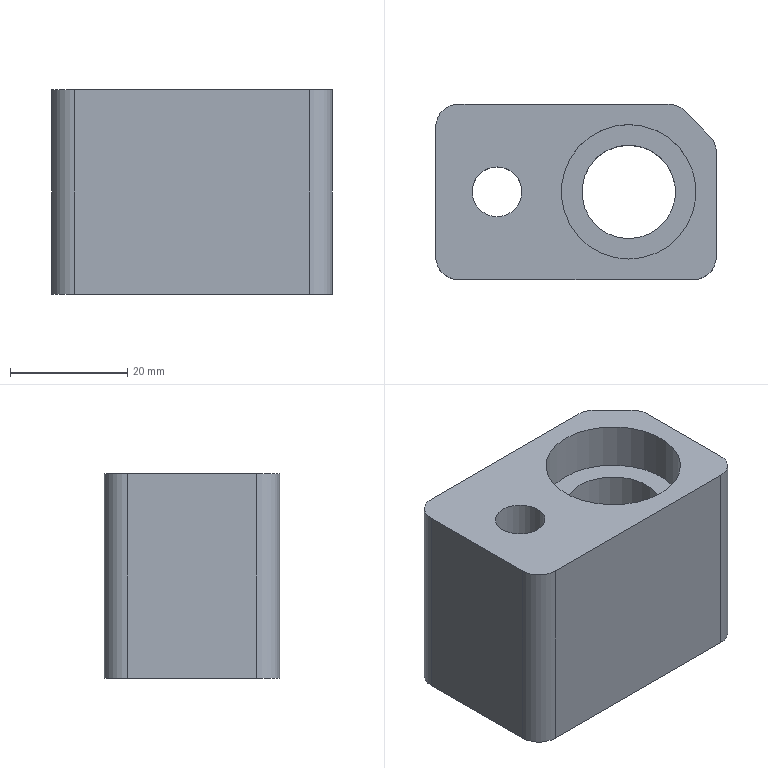Part | NX | features 7 2 | 1 solid | 18 faces | box 48 x 30 x 35 mm | volume 36880 mm3 | plane 9 | cylinder 9 | commonest cylinder face diameters 8 x5 8.5 x1 14.5 x1 16 x1 23 x1
STEP:
#1=CARTESIAN_POINT('',(21.306,11.5,91.));
#2=VERTEX_POINT('',#1);
#3=CARTESIAN_POINT('',(21.306,0.,91.));
#4=DIRECTION('',(0.,0.,-1.));
#5=DIRECTION('',(0.,1.,0.));
#6=AXIS2_PLACEMENT_3D('',#3,#4,#5);
#7=CIRCLE('',#6,11.5);
#8=EDGE_CURVE('',#2,#2,#7,.T.);
#9=ORIENTED_EDGE('',*,*,#8,.T.);
#10=EDGE_LOOP('',(#9));
#11=FACE_BOUND('',#10,.T.);
#12=CARTESIAN_POINT('',(-7.694,-15.,91.));
#13=VERTEX_POINT('',#12);
#14=CARTESIAN_POINT('',(32.306,-15.,91.));
#15=VERTEX_POINT('',#14);
#16=CARTESIAN_POINT('',(21.306,-15.,91.));
#17=DIRECTION('',(1.,0.,0.));
#18=VECTOR('',#17,1000.);
#19=LINE('',#16,#18);
#20=EDGE_CURVE('',#13,#15,#19,.T.);
#21=ORIENTED_EDGE('',*,*,#20,.T.);
#22=CARTESIAN_POINT('',(36.306,-11.,91.));
#23=VERTEX_POINT('',#22);
#24=CARTESIAN_POINT('',(32.306,-11.,91.));
#25=DIRECTION('',(0.,0.,-1.));
#26=DIRECTION('',(0.,1.,0.));
#27=AXIS2_PLACEMENT_3D('',#24,#25,#26);
#28=CIRCLE('',#27,4.);
#29=EDGE_CURVE('',#23,#15,#28,.T.);
#30=ORIENTED_EDGE('',*,*,#29,.F.);
#31=CARTESIAN_POINT('',(36.306,6.707,91.));
#32=VERTEX_POINT('',#31);
#33=CARTESIAN_POINT('',(36.306,0.,91.));
#34=DIRECTION('',(0.,1.,0.));
#35=VECTOR('',#34,1000.);
#36=LINE('',#33,#35);
#37=EDGE_CURVE('',#23,#32,#36,.T.);
#38=ORIENTED_EDGE('',*,*,#37,.T.);
#39=CARTESIAN_POINT('',(35.135,9.536,91.));
#40=VERTEX_POINT('',#39);
#41=CARTESIAN_POINT('',(32.306,6.707,91.));
#42=DIRECTION('',(0.,0.,-1.));
#43=DIRECTION('',(0.,1.,0.));
#44=AXIS2_PLACEMENT_3D('',#41,#42,#43);
#45=CIRCLE('',#44,4.);
#46=EDGE_CURVE('',#40,#32,#45,.T.);
#47=ORIENTED_EDGE('',*,*,#46,.F.);
#48=CARTESIAN_POINT('',(30.842,13.828,91.));
#49=VERTEX_POINT('',#48);
#50=CARTESIAN_POINT('',(31.738,12.932,91.));
#51=DIRECTION('',(0.7071,-0.7071,0.));
#52=VECTOR('',#51,1000.);
#53=LINE('',#50,#52);
#54=EDGE_CURVE('',#49,#40,#53,.T.);
#55=ORIENTED_EDGE('',*,*,#54,.F.);
#56=CARTESIAN_POINT('',(28.013,15.,91.));
#57=VERTEX_POINT('',#56);
#58=CARTESIAN_POINT('',(28.013,11.,91.));
#59=DIRECTION('',(0.,0.,-1.));
#60=DIRECTION('',(0.,1.,0.));
#61=AXIS2_PLACEMENT_3D('',#58,#59,#60);
#62=CIRCLE('',#61,4.);
#63=EDGE_CURVE('',#57,#49,#62,.T.);
#64=ORIENTED_EDGE('',*,*,#63,.F.);
#65=CARTESIAN_POINT('',(-7.694,15.,91.));
#66=VERTEX_POINT('',#65);
#67=CARTESIAN_POINT('',(21.306,15.,91.));
#68=DIRECTION('',(-1.,0.,0.));
#69=VECTOR('',#68,1000.);
#70=LINE('',#67,#69);
#71=EDGE_CURVE('',#57,#66,#70,.T.);
#72=ORIENTED_EDGE('',*,*,#71,.T.);
#73=CARTESIAN_POINT('',(-11.694,11.,91.));
#74=VERTEX_POINT('',#73);
#75=CARTESIAN_POINT('',(-7.694,11.,91.));
#76=DIRECTION('',(0.,0.,-1.));
#77=DIRECTION('',(0.,1.,0.));
#78=AXIS2_PLACEMENT_3D('',#75,#76,#77);
#79=CIRCLE('',#78,4.);
#80=EDGE_CURVE('',#74,#66,#79,.T.);
#81=ORIENTED_EDGE('',*,*,#80,.F.);
#82=CARTESIAN_POINT('',(-11.694,-11.,91.));
#83=VERTEX_POINT('',#82);
#84=CARTESIAN_POINT('',(-11.694,0.,91.));
#85=DIRECTION('',(0.,-1.,0.));
#86=VECTOR('',#85,1000.);
#87=LINE('',#84,#86);
#88=EDGE_CURVE('',#74,#83,#87,.T.);
#89=ORIENTED_EDGE('',*,*,#88,.T.);
#90=CARTESIAN_POINT('',(-7.694,-11.,91.));
#91=DIRECTION('',(0.,0.,-1.));
#92=DIRECTION('',(0.,1.,0.));
#93=AXIS2_PLACEMENT_3D('',#90,#91,#92);
#94=CIRCLE('',#93,4.);
#95=EDGE_CURVE('',#13,#83,#94,.T.);
#96=ORIENTED_EDGE('',*,*,#95,.F.);
#97=EDGE_LOOP('',(#21,#30,#38,#47,#55,#64,#72,#81,#89,#96));
#98=FACE_BOUND('',#97,.T.);
#99=CARTESIAN_POINT('',(-1.194,4.25,91.));
#100=VERTEX_POINT('',#99);
#101=CARTESIAN_POINT('',(-1.194,0.,91.));
#102=DIRECTION('',(0.,0.,1.));
#103=DIRECTION('',(0.,1.,0.));
#104=AXIS2_PLACEMENT_3D('',#101,#102,#103);
#105=CIRCLE('',#104,4.25);
#106=EDGE_CURVE('',#100,#100,#105,.T.);
#107=ORIENTED_EDGE('',*,*,#106,.F.);
#108=EDGE_LOOP('',(#107));
#109=FACE_BOUND('',#108,.T.);
#110=CARTESIAN_POINT('',(18.806,0.,91.));
#111=DIRECTION('',(0.,0.,1.));
#112=DIRECTION('',(0.,-1.,0.));
#113=AXIS2_PLACEMENT_3D('',#110,#111,#112);
#114=PLANE('',#113);
#115=ADVANCED_FACE('',(#11,#98,#109),#114,.T.);
#116=CARTESIAN_POINT('',(21.306,-8.,56.));
#117=VERTEX_POINT('',#116);
#118=CARTESIAN_POINT('',(21.306,0.,56.));
#119=DIRECTION('',(0.,0.,1.));
#120=DIRECTION('',(0.,-1.,0.));
#121=AXIS2_PLACEMENT_3D('',#118,#119,#120);
#122=CIRCLE('',#121,8.);
#123=EDGE_CURVE('',#117,#117,#122,.T.);
#124=ORIENTED_EDGE('',*,*,#123,.T.);
#125=EDGE_LOOP('',(#124));
#126=FACE_BOUND('',#125,.T.);
#127=CARTESIAN_POINT('',(-1.194,-7.25,56.));
#128=VERTEX_POINT('',#127);
#129=CARTESIAN_POINT('',(-1.194,0.,56.));
#130=DIRECTION('',(0.,0.,1.));
#131=DIRECTION('',(0.,-1.,0.));
#132=AXIS2_PLACEMENT_3D('',#129,#130,#131);
#133=CIRCLE('',#132,7.25);
#134=EDGE_CURVE('',#128,#128,#133,.T.);
#135=ORIENTED_EDGE('',*,*,#134,.T.);
#136=EDGE_LOOP('',(#135));
#137=FACE_BOUND('',#136,.T.);
#138=CARTESIAN_POINT('',(-11.694,-11.,56.));
#139=VERTEX_POINT('',#138);
#140=CARTESIAN_POINT('',(-11.694,11.,56.));
#141=VERTEX_POINT('',#140);
#142=CARTESIAN_POINT('',(-11.694,0.,56.));
#143=DIRECTION('',(0.,1.,0.));
#144=VECTOR('',#143,1000.);
#145=LINE('',#142,#144);
#146=EDGE_CURVE('',#139,#141,#145,.T.);
#147=ORIENTED_EDGE('',*,*,#146,.T.);
#148=CARTESIAN_POINT('',(-7.694,15.,56.));
#149=VERTEX_POINT('',#148);
#150=CARTESIAN_POINT('',(-7.694,11.,56.));
#151=DIRECTION('',(0.,0.,1.));
#152=DIRECTION('',(0.,-1.,0.));
#153=AXIS2_PLACEMENT_3D('',#150,#151,#152);
#154=CIRCLE('',#153,4.);
#155=EDGE_CURVE('',#149,#141,#154,.T.);
#156=ORIENTED_EDGE('',*,*,#155,.F.);
#157=CARTESIAN_POINT('',(28.013,15.,56.));
#158=VERTEX_POINT('',#157);
#159=CARTESIAN_POINT('',(21.306,15.,56.));
#160=DIRECTION('',(1.,0.,0.));
#161=VECTOR('',#160,1000.);
#162=LINE('',#159,#161);
#163=EDGE_CURVE('',#149,#158,#162,.T.);
#164=ORIENTED_EDGE('',*,*,#163,.T.);
#165=CARTESIAN_POINT('',(30.842,13.828,56.));
#166=VERTEX_POINT('',#165);
#167=CARTESIAN_POINT('',(28.013,11.,56.));
#168=DIRECTION('',(0.,0.,1.));
#169=DIRECTION('',(0.,-1.,0.));
#170=AXIS2_PLACEMENT_3D('',#167,#168,#169);
#171=CIRCLE('',#170,4.);
#172=EDGE_CURVE('',#166,#158,#171,.T.);
#173=ORIENTED_EDGE('',*,*,#172,.F.);
#174=CARTESIAN_POINT('',(35.135,9.536,56.));
#175=VERTEX_POINT('',#174);
#176=CARTESIAN_POINT('',(28.988,15.682,56.));
#177=DIRECTION('',(-0.7071,0.7071,0.));
#178=VECTOR('',#177,1000.);
#179=LINE('',#176,#178);
#180=EDGE_CURVE('',#175,#166,#179,.T.);
#181=ORIENTED_EDGE('',*,*,#180,.F.);
#182=CARTESIAN_POINT('',(36.306,6.707,56.));
#183=VERTEX_POINT('',#182);
#184=CARTESIAN_POINT('',(32.306,6.707,56.));
#185=DIRECTION('',(0.,0.,1.));
#186=DIRECTION('',(0.,-1.,0.));
#187=AXIS2_PLACEMENT_3D('',#184,#185,#186);
#188=CIRCLE('',#187,4.);
#189=EDGE_CURVE('',#183,#175,#188,.T.);
#190=ORIENTED_EDGE('',*,*,#189,.F.);
#191=CARTESIAN_POINT('',(36.306,-11.,56.));
#192=VERTEX_POINT('',#191);
#193=CARTESIAN_POINT('',(36.306,0.,56.));
#194=DIRECTION('',(0.,-1.,0.));
#195=VECTOR('',#194,1000.);
#196=LINE('',#193,#195);
#197=EDGE_CURVE('',#183,#192,#196,.T.);
#198=ORIENTED_EDGE('',*,*,#197,.T.);
#199=CARTESIAN_POINT('',(32.306,-15.,56.));
#200=VERTEX_POINT('',#199);
#201=CARTESIAN_POINT('',(32.306,-11.,56.));
#202=DIRECTION('',(0.,0.,1.));
#203=DIRECTION('',(0.,-1.,0.));
#204=AXIS2_PLACEMENT_3D('',#201,#202,#203);
#205=CIRCLE('',#204,4.);
#206=EDGE_CURVE('',#200,#192,#205,.T.);
#207=ORIENTED_EDGE('',*,*,#206,.F.);
#208=CARTESIAN_POINT('',(-7.694,-15.,56.));
#209=VERTEX_POINT('',#208);
#210=CARTESIAN_POINT('',(21.306,-15.,56.));
#211=DIRECTION('',(-1.,0.,0.));
#212=VECTOR('',#211,1000.);
#213=LINE('',#210,#212);
#214=EDGE_CURVE('',#200,#209,#213,.T.);
#215=ORIENTED_EDGE('',*,*,#214,.T.);
#216=CARTESIAN_POINT('',(-7.694,-11.,56.));
#217=DIRECTION('',(0.,0.,1.));
#218=DIRECTION('',(0.,-1.,0.));
#219=AXIS2_PLACEMENT_3D('',#216,#217,#218);
#220=CIRCLE('',#219,4.);
#221=EDGE_CURVE('',#139,#209,#220,.T.);
#222=ORIENTED_EDGE('',*,*,#221,.F.);
#223=EDGE_LOOP('',(#147,#156,#164,#173,#181,#190,#198,#207,#215,#222));
#224=FACE_BOUND('',#223,.T.);
#225=CARTESIAN_POINT('',(-163.694,-177.,56.));
#226=DIRECTION('',(0.,0.,-1.));
#227=DIRECTION('',(0.,1.,0.));
#228=AXIS2_PLACEMENT_3D('',#225,#226,#227);
#229=PLANE('',#228);
#230=ADVANCED_FACE('',(#126,#137,#224),#229,.T.);
#231=ORIENTED_EDGE('',*,*,#37,.F.);
#232=CARTESIAN_POINT('',(36.306,-11.,-5.));
#233=DIRECTION('',(0.,0.,1.));
#234=VECTOR('',#233,1000.);
#235=LINE('',#232,#234);
#236=EDGE_CURVE('',#192,#23,#235,.T.);
#237=ORIENTED_EDGE('',*,*,#236,.F.);
#238=ORIENTED_EDGE('',*,*,#197,.F.);
#239=CARTESIAN_POINT('',(36.306,6.707,-5.));
#240=DIRECTION('',(0.,0.,-1.));
#241=VECTOR('',#240,1000.);
#242=LINE('',#239,#241);
#243=EDGE_CURVE('',#32,#183,#242,.T.);
#244=ORIENTED_EDGE('',*,*,#243,.F.);
#245=EDGE_LOOP('',(#231,#237,#238,#244));
#246=FACE_BOUND('',#245,.T.);
#247=CARTESIAN_POINT('',(36.306,0.,-5.));
#248=DIRECTION('',(1.,0.,0.));
#249=DIRECTION('',(0.,0.,-1.));
#250=AXIS2_PLACEMENT_3D('',#247,#248,#249);
#251=PLANE('',#250);
#252=ADVANCED_FACE('',(#246),#251,.T.);
#253=ORIENTED_EDGE('',*,*,#71,.F.);
#254=CARTESIAN_POINT('',(28.013,15.,-5.));
#255=DIRECTION('',(0.,0.,1.));
#256=VECTOR('',#255,1000.);
#257=LINE('',#254,#256);
#258=EDGE_CURVE('',#158,#57,#257,.T.);
#259=ORIENTED_EDGE('',*,*,#258,.F.);
#260=ORIENTED_EDGE('',*,*,#163,.F.);
#261=CARTESIAN_POINT('',(-7.694,15.,-5.));
#262=DIRECTION('',(0.,0.,-1.));
#263=VECTOR('',#262,1000.);
#264=LINE('',#261,#263);
#265=EDGE_CURVE('',#66,#149,#264,.T.);
#266=ORIENTED_EDGE('',*,*,#265,.F.);
#267=EDGE_LOOP('',(#253,#259,#260,#266));
#268=FACE_BOUND('',#267,.T.);
#269=CARTESIAN_POINT('',(21.306,15.,-5.));
#270=DIRECTION('',(0.,1.,0.));
#271=DIRECTION('',(0.,0.,1.));
#272=AXIS2_PLACEMENT_3D('',#269,#270,#271);
#273=PLANE('',#272);
#274=ADVANCED_FACE('',(#268),#273,.T.);
#275=ORIENTED_EDGE('',*,*,#88,.F.);
#276=CARTESIAN_POINT('',(-11.694,11.,-5.));
#277=DIRECTION('',(0.,0.,1.));
#278=VECTOR('',#277,1000.);
#279=LINE('',#276,#278);
#280=EDGE_CURVE('',#141,#74,#279,.T.);
#281=ORIENTED_EDGE('',*,*,#280,.F.);
#282=ORIENTED_EDGE('',*,*,#146,.F.);
#283=CARTESIAN_POINT('',(-11.694,-11.,-5.));
#284=DIRECTION('',(0.,0.,-1.));
#285=VECTOR('',#284,1000.);
#286=LINE('',#283,#285);
#287=EDGE_CURVE('',#83,#139,#286,.T.);
#288=ORIENTED_EDGE('',*,*,#287,.F.);
#289=EDGE_LOOP('',(#275,#281,#282,#288));
#290=FACE_BOUND('',#289,.T.);
#291=CARTESIAN_POINT('',(-11.694,0.,-5.));
#292=DIRECTION('',(-1.,0.,0.));
#293=DIRECTION('',(0.,0.,1.));
#294=AXIS2_PLACEMENT_3D('',#291,#292,#293);
#295=PLANE('',#294);
#296=ADVANCED_FACE('',(#290),#295,.T.);
#297=ORIENTED_EDGE('',*,*,#214,.F.);
#298=CARTESIAN_POINT('',(32.306,-15.,-5.));
#299=DIRECTION('',(0.,0.,-1.));
#300=VECTOR('',#299,1000.);
#301=LINE('',#298,#300);
#302=EDGE_CURVE('',#15,#200,#301,.T.);
#303=ORIENTED_EDGE('',*,*,#302,.F.);
#304=ORIENTED_EDGE('',*,*,#20,.F.);
#305=CARTESIAN_POINT('',(-7.694,-15.,-5.));
#306=DIRECTION('',(0.,0.,1.));
#307=VECTOR('',#306,1000.);
#308=LINE('',#305,#307);
#309=EDGE_CURVE('',#209,#13,#308,.T.);
#310=ORIENTED_EDGE('',*,*,#309,.F.);
#311=EDGE_LOOP('',(#297,#303,#304,#310));
#312=FACE_BOUND('',#311,.T.);
#313=CARTESIAN_POINT('',(21.306,-15.,-5.));
#314=DIRECTION('',(0.,-1.,0.));
#315=DIRECTION('',(0.,0.,-1.));
#316=AXIS2_PLACEMENT_3D('',#313,#314,#315);
#317=PLANE('',#316);
#318=ADVANCED_FACE('',(#312),#317,.T.);
#319=ORIENTED_EDGE('',*,*,#54,.T.);
#320=CARTESIAN_POINT('',(35.135,9.536,-5.));
#321=DIRECTION('',(0.,0.,1.));
#322=VECTOR('',#321,1000.);
#323=LINE('',#320,#322);
#324=EDGE_CURVE('',#175,#40,#323,.T.);
#325=ORIENTED_EDGE('',*,*,#324,.F.);
#326=ORIENTED_EDGE('',*,*,#180,.T.);
#327=CARTESIAN_POINT('',(30.842,13.828,-5.));
#328=DIRECTION('',(0.,0.,-1.));
#329=VECTOR('',#328,1000.);
#330=LINE('',#327,#329);
#331=EDGE_CURVE('',#49,#166,#330,.T.);
#332=ORIENTED_EDGE('',*,*,#331,.F.);
#333=EDGE_LOOP('',(#319,#325,#326,#332));
#334=FACE_BOUND('',#333,.T.);
#335=CARTESIAN_POINT('',(28.988,15.682,-5.));
#336=DIRECTION('',(-0.7071,-0.7071,0.));
#337=DIRECTION('',(0.,0.,1.));
#338=AXIS2_PLACEMENT_3D('',#335,#336,#337);
#339=PLANE('',#338);
#340=ADVANCED_FACE('',(#334),#339,.F.);
#341=ORIENTED_EDGE('',*,*,#221,.T.);
#342=ORIENTED_EDGE('',*,*,#309,.T.);
#343=ORIENTED_EDGE('',*,*,#95,.T.);
#344=ORIENTED_EDGE('',*,*,#287,.T.);
#345=EDGE_LOOP('',(#341,#342,#343,#344));
#346=FACE_BOUND('',#345,.T.);
#347=CARTESIAN_POINT('',(-7.694,-11.,-5.));
#348=DIRECTION('',(0.,0.,-1.));
#349=DIRECTION('',(0.,-1.,0.));
#350=AXIS2_PLACEMENT_3D('',#347,#348,#349);
#351=CYLINDRICAL_SURFACE('',#350,4.);
#352=ADVANCED_FACE('',(#346),#351,.T.);
#353=ORIENTED_EDGE('',*,*,#155,.T.);
#354=ORIENTED_EDGE('',*,*,#280,.T.);
#355=ORIENTED_EDGE('',*,*,#80,.T.);
#356=ORIENTED_EDGE('',*,*,#265,.T.);
#357=EDGE_LOOP('',(#353,#354,#355,#356));
#358=FACE_BOUND('',#357,.T.);
#359=CARTESIAN_POINT('',(-7.694,11.,-5.));
#360=DIRECTION('',(0.,0.,-1.));
#361=DIRECTION('',(0.,-1.,0.));
#362=AXIS2_PLACEMENT_3D('',#359,#360,#361);
#363=CYLINDRICAL_SURFACE('',#362,4.);
#364=ADVANCED_FACE('',(#358),#363,.T.);
#365=ORIENTED_EDGE('',*,*,#172,.T.);
#366=ORIENTED_EDGE('',*,*,#258,.T.);
#367=ORIENTED_EDGE('',*,*,#63,.T.);
#368=ORIENTED_EDGE('',*,*,#331,.T.);
#369=EDGE_LOOP('',(#365,#366,#367,#368));
#370=FACE_BOUND('',#369,.T.);
#371=CARTESIAN_POINT('',(28.013,11.,-5.));
#372=DIRECTION('',(0.,0.,1.));
#373=DIRECTION('',(0.,1.,0.));
#374=AXIS2_PLACEMENT_3D('',#371,#372,#373);
#375=CYLINDRICAL_SURFACE('',#374,4.);
#376=ADVANCED_FACE('',(#370),#375,.T.);
#377=ORIENTED_EDGE('',*,*,#46,.T.);
#378=ORIENTED_EDGE('',*,*,#243,.T.);
#379=ORIENTED_EDGE('',*,*,#189,.T.);
#380=ORIENTED_EDGE('',*,*,#324,.T.);
#381=EDGE_LOOP('',(#377,#378,#379,#380));
#382=FACE_BOUND('',#381,.T.);
#383=CARTESIAN_POINT('',(32.306,6.707,-5.));
#384=DIRECTION('',(0.,0.,-1.));
#385=DIRECTION('',(0.,-1.,0.));
#386=AXIS2_PLACEMENT_3D('',#383,#384,#385);
#387=CYLINDRICAL_SURFACE('',#386,4.);
#388=ADVANCED_FACE('',(#382),#387,.T.);
#389=ORIENTED_EDGE('',*,*,#206,.T.);
#390=ORIENTED_EDGE('',*,*,#236,.T.);
#391=ORIENTED_EDGE('',*,*,#29,.T.);
#392=ORIENTED_EDGE('',*,*,#302,.T.);
#393=EDGE_LOOP('',(#389,#390,#391,#392));
#394=FACE_BOUND('',#393,.T.);
#395=CARTESIAN_POINT('',(32.306,-11.,-5.));
#396=DIRECTION('',(0.,0.,-1.));
#397=DIRECTION('',(0.,-1.,0.));
#398=AXIS2_PLACEMENT_3D('',#395,#396,#397);
#399=CYLINDRICAL_SURFACE('',#398,4.);
#400=ADVANCED_FACE('',(#394),#399,.T.);
#401=CARTESIAN_POINT('',(-1.194,4.25,71.));
#402=VERTEX_POINT('',#401);
#403=CARTESIAN_POINT('',(-1.194,0.,71.));
#404=DIRECTION('',(0.,0.,-1.));
#405=DIRECTION('',(0.,1.,0.));
#406=AXIS2_PLACEMENT_3D('',#403,#404,#405);
#407=CIRCLE('',#406,4.25);
#408=EDGE_CURVE('',#402,#402,#407,.T.);
#409=ORIENTED_EDGE('',*,*,#408,.T.);
#410=EDGE_LOOP('',(#409));
#411=FACE_BOUND('',#410,.T.);
#412=ORIENTED_EDGE('',*,*,#106,.T.);
#413=EDGE_LOOP('',(#412));
#414=FACE_BOUND('',#413,.T.);
#415=CARTESIAN_POINT('',(-1.194,0.,55.));
#416=DIRECTION('',(0.,0.,1.));
#417=DIRECTION('',(0.,-1.,0.));
#418=AXIS2_PLACEMENT_3D('',#415,#416,#417);
#419=CYLINDRICAL_SURFACE('',#418,4.25);
#420=ADVANCED_FACE('',(#411,#414),#419,.F.);
#421=ORIENTED_EDGE('',*,*,#408,.F.);
#422=EDGE_LOOP('',(#421));
#423=FACE_BOUND('',#422,.T.);
#424=CARTESIAN_POINT('',(-1.194,7.25,71.));
#425=VERTEX_POINT('',#424);
#426=CARTESIAN_POINT('',(-1.194,0.,71.));
#427=DIRECTION('',(0.,0.,-1.));
#428=DIRECTION('',(0.,1.,0.));
#429=AXIS2_PLACEMENT_3D('',#426,#427,#428);
#430=CIRCLE('',#429,7.25);
#431=EDGE_CURVE('',#425,#425,#430,.T.);
#432=ORIENTED_EDGE('',*,*,#431,.T.);
#433=EDGE_LOOP('',(#432));
#434=FACE_BOUND('',#433,.T.);
#435=CARTESIAN_POINT('',(-1.194,0.,71.));
#436=DIRECTION('',(0.,0.,1.));
#437=DIRECTION('',(0.,-1.,0.));
#438=AXIS2_PLACEMENT_3D('',#435,#436,#437);
#439=PLANE('',#438);
#440=ADVANCED_FACE('',(#423,#434),#439,.F.);
#441=ORIENTED_EDGE('',*,*,#134,.F.);
#442=EDGE_LOOP('',(#441));
#443=FACE_BOUND('',#442,.T.);
#444=ORIENTED_EDGE('',*,*,#431,.F.);
#445=EDGE_LOOP('',(#444));
#446=FACE_BOUND('',#445,.T.);
#447=CARTESIAN_POINT('',(-1.194,0.,55.));
#448=DIRECTION('',(0.,0.,1.));
#449=DIRECTION('',(0.,-1.,0.));
#450=AXIS2_PLACEMENT_3D('',#447,#448,#449);
#451=CYLINDRICAL_SURFACE('',#450,7.25);
#452=ADVANCED_FACE('',(#443,#446),#451,.F.);
#453=CARTESIAN_POINT('',(21.306,-8.,83.));
#454=VERTEX_POINT('',#453);
#455=CARTESIAN_POINT('',(21.306,0.,83.));
#456=DIRECTION('',(0.,0.,-1.));
#457=DIRECTION('',(0.,-1.,0.));
#458=AXIS2_PLACEMENT_3D('',#455,#456,#457);
#459=CIRCLE('',#458,8.);
#460=EDGE_CURVE('',#454,#454,#459,.T.);
#461=ORIENTED_EDGE('',*,*,#460,.F.);
#462=EDGE_LOOP('',(#461));
#463=FACE_BOUND('',#462,.T.);
#464=ORIENTED_EDGE('',*,*,#123,.F.);
#465=EDGE_LOOP('',(#464));
#466=FACE_BOUND('',#465,.T.);
#467=CARTESIAN_POINT('',(21.306,0.,91.));
#468=DIRECTION('',(0.,0.,-1.));
#469=DIRECTION('',(0.,-1.,0.));
#470=AXIS2_PLACEMENT_3D('',#467,#468,#469);
#471=CYLINDRICAL_SURFACE('',#470,8.);
#472=ADVANCED_FACE('',(#463,#466),#471,.F.);
#473=CARTESIAN_POINT('',(21.306,-11.5,83.));
#474=VERTEX_POINT('',#473);
#475=CARTESIAN_POINT('',(21.306,0.,83.));
#476=DIRECTION('',(0.,0.,1.));
#477=DIRECTION('',(0.,-1.,0.));
#478=AXIS2_PLACEMENT_3D('',#475,#476,#477);
#479=CIRCLE('',#478,11.5);
#480=EDGE_CURVE('',#474,#474,#479,.T.);
#481=ORIENTED_EDGE('',*,*,#480,.T.);
#482=EDGE_LOOP('',(#481));
#483=FACE_BOUND('',#482,.T.);
#484=ORIENTED_EDGE('',*,*,#460,.T.);
#485=EDGE_LOOP('',(#484));
#486=FACE_BOUND('',#485,.T.);
#487=CARTESIAN_POINT('',(21.306,0.,83.));
#488=DIRECTION('',(0.,0.,-1.));
#489=DIRECTION('',(0.,-1.,0.));
#490=AXIS2_PLACEMENT_3D('',#487,#488,#489);
#491=PLANE('',#490);
#492=ADVANCED_FACE('',(#483,#486),#491,.F.);
#493=ORIENTED_EDGE('',*,*,#8,.F.);
#494=EDGE_LOOP('',(#493));
#495=FACE_BOUND('',#494,.T.);
#496=ORIENTED_EDGE('',*,*,#480,.F.);
#497=EDGE_LOOP('',(#496));
#498=FACE_BOUND('',#497,.T.);
#499=CARTESIAN_POINT('',(21.306,0.,90.559));
#500=DIRECTION('',(0.,0.,-1.));
#501=DIRECTION('',(0.,1.,0.));
#502=AXIS2_PLACEMENT_3D('',#499,#500,#501);
#503=CYLINDRICAL_SURFACE('',#502,11.5);
#504=ADVANCED_FACE('',(#495,#498),#503,.F.);
#505=CLOSED_SHELL('',(#115,#230,#252,#274,#296,#318,#340,#352,#364,#376,#388,#400,#420,#440,#452,#472,#492,#504));
#506=MANIFOLD_SOLID_BREP('',#505);
#507=(LENGTH_UNIT()NAMED_UNIT(*)SI_UNIT(.MILLI.,.METRE.));
#508=UNCERTAINTY_MEASURE_WITH_UNIT(LENGTH_MEASURE(0.00001),#507,'','');
#509=(NAMED_UNIT(*)PLANE_ANGLE_UNIT()SI_UNIT($,.RADIAN.));
#510=(NAMED_UNIT(*)SI_UNIT($,.STERADIAN.)SOLID_ANGLE_UNIT());
#511=(GEOMETRIC_REPRESENTATION_CONTEXT(3)GLOBAL_UNCERTAINTY_ASSIGNED_CONTEXT((#508))GLOBAL_UNIT_ASSIGNED_CONTEXT((#507,#509,#510))REPRESENTATION_CONTEXT('',''));
#512=ADVANCED_BREP_SHAPE_REPRESENTATION('',(#506),#511);